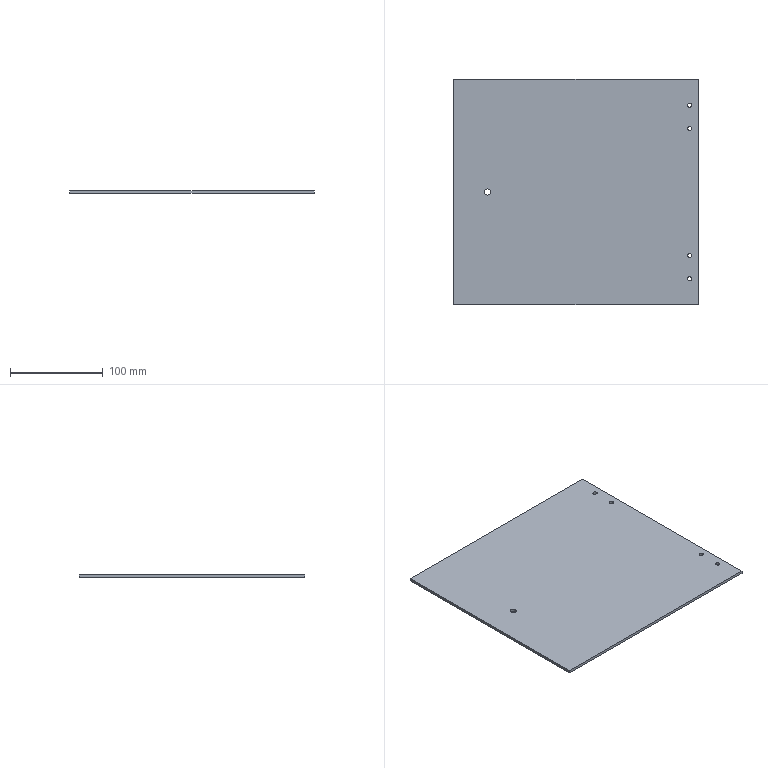Part | SolidWorks | features Cut 2, Extrusion 1, MirrorPattern 1 | 1 solid | 16 faces | box 263 x 243 x 3 mm | volume 191442 mm3 | cylinder 10 | plane 6 | commonest cylinder face diameters 4.4 x8 6.6 x2
STEP:
#1=CARTESIAN_POINT('',(-98.8,0.,0.));
#2=VERTEX_POINT('',#1);
#3=CARTESIAN_POINT('',(-92.2,0.,0.));
#4=VERTEX_POINT('',#3);
#5=CARTESIAN_POINT('',(-95.5,0.,0.));
#6=DIRECTION('',(0.,0.,1.));
#7=DIRECTION('',(1.,0.,0.));
#8=AXIS2_PLACEMENT_3D('',#5,#6,#7);
#9=CIRCLE('',#8,3.3);
#10=EDGE_CURVE('',#2,#4,#9,.T.);
#11=ORIENTED_EDGE('',*,*,#10,.F.);
#12=CARTESIAN_POINT('',(-98.8,0.,3.));
#13=VERTEX_POINT('',#12);
#14=CARTESIAN_POINT('',(-98.8,0.,-7.));
#15=DIRECTION('',(0.,0.,1.));
#16=VECTOR('',#15,1000.);
#17=LINE('',#14,#16);
#18=EDGE_CURVE('',#2,#13,#17,.T.);
#19=ORIENTED_EDGE('',*,*,#18,.T.);
#20=CARTESIAN_POINT('',(-92.2,0.,3.));
#21=VERTEX_POINT('',#20);
#22=CARTESIAN_POINT('',(-95.5,0.,3.));
#23=DIRECTION('',(0.,0.,1.));
#24=DIRECTION('',(1.,0.,0.));
#25=AXIS2_PLACEMENT_3D('',#22,#23,#24);
#26=CIRCLE('',#25,3.3);
#27=EDGE_CURVE('',#13,#21,#26,.T.);
#28=ORIENTED_EDGE('',*,*,#27,.T.);
#29=CARTESIAN_POINT('',(-92.2,0.,-7.));
#30=DIRECTION('',(0.,0.,1.));
#31=VECTOR('',#30,1000.);
#32=LINE('',#29,#31);
#33=EDGE_CURVE('',#4,#21,#32,.T.);
#34=ORIENTED_EDGE('',*,*,#33,.F.);
#35=EDGE_LOOP('',(#11,#19,#28,#34));
#36=FACE_OUTER_BOUND('',#35,.T.);
#37=CARTESIAN_POINT('',(-95.5,0.,-7.));
#38=DIRECTION('',(0.,0.,1.));
#39=DIRECTION('',(1.,0.,0.));
#40=AXIS2_PLACEMENT_3D('',#37,#38,#39);
#41=CYLINDRICAL_SURFACE('',#40,3.3);
#42=ADVANCED_FACE('',(#36),#41,.F.);
#43=CARTESIAN_POINT('',(124.7,68.5,3.));
#44=VERTEX_POINT('',#43);
#45=CARTESIAN_POINT('',(120.3,68.5,3.));
#46=VERTEX_POINT('',#45);
#47=CARTESIAN_POINT('',(122.5,68.5,3.));
#48=DIRECTION('',(0.,0.,-1.));
#49=DIRECTION('',(1.,0.,0.));
#50=AXIS2_PLACEMENT_3D('',#47,#48,#49);
#51=CIRCLE('',#50,2.2);
#52=EDGE_CURVE('',#44,#46,#51,.T.);
#53=ORIENTED_EDGE('',*,*,#52,.F.);
#54=CARTESIAN_POINT('',(124.7,68.5,0.));
#55=VERTEX_POINT('',#54);
#56=CARTESIAN_POINT('',(124.7,68.5,10.));
#57=DIRECTION('',(0.,0.,-1.));
#58=VECTOR('',#57,1000.);
#59=LINE('',#56,#58);
#60=EDGE_CURVE('',#44,#55,#59,.T.);
#61=ORIENTED_EDGE('',*,*,#60,.T.);
#62=CARTESIAN_POINT('',(120.3,68.5,0.));
#63=VERTEX_POINT('',#62);
#64=CARTESIAN_POINT('',(122.5,68.5,0.));
#65=DIRECTION('',(0.,0.,1.));
#66=DIRECTION('',(-1.,0.,0.));
#67=AXIS2_PLACEMENT_3D('',#64,#65,#66);
#68=CIRCLE('',#67,2.2);
#69=EDGE_CURVE('',#63,#55,#68,.T.);
#70=ORIENTED_EDGE('',*,*,#69,.F.);
#71=CARTESIAN_POINT('',(120.3,68.5,10.));
#72=DIRECTION('',(0.,0.,-1.));
#73=VECTOR('',#72,1000.);
#74=LINE('',#71,#73);
#75=EDGE_CURVE('',#46,#63,#74,.T.);
#76=ORIENTED_EDGE('',*,*,#75,.F.);
#77=EDGE_LOOP('',(#53,#61,#70,#76));
#78=FACE_OUTER_BOUND('',#77,.T.);
#79=CARTESIAN_POINT('',(122.5,68.5,10.));
#80=DIRECTION('',(0.,0.,-1.));
#81=DIRECTION('',(-1.,0.,0.));
#82=AXIS2_PLACEMENT_3D('',#79,#80,#81);
#83=CYLINDRICAL_SURFACE('',#82,2.2);
#84=ADVANCED_FACE('',(#78),#83,.F.);
#85=CARTESIAN_POINT('',(124.7,93.5,3.));
#86=VERTEX_POINT('',#85);
#87=CARTESIAN_POINT('',(120.3,93.5,3.));
#88=VERTEX_POINT('',#87);
#89=CARTESIAN_POINT('',(122.5,93.5,3.));
#90=DIRECTION('',(0.,0.,-1.));
#91=DIRECTION('',(1.,0.,0.));
#92=AXIS2_PLACEMENT_3D('',#89,#90,#91);
#93=CIRCLE('',#92,2.2);
#94=EDGE_CURVE('',#86,#88,#93,.T.);
#95=ORIENTED_EDGE('',*,*,#94,.F.);
#96=CARTESIAN_POINT('',(124.7,93.5,0.));
#97=VERTEX_POINT('',#96);
#98=CARTESIAN_POINT('',(124.7,93.5,10.));
#99=DIRECTION('',(0.,0.,-1.));
#100=VECTOR('',#99,1000.);
#101=LINE('',#98,#100);
#102=EDGE_CURVE('',#86,#97,#101,.T.);
#103=ORIENTED_EDGE('',*,*,#102,.T.);
#104=CARTESIAN_POINT('',(120.3,93.5,0.));
#105=VERTEX_POINT('',#104);
#106=CARTESIAN_POINT('',(122.5,93.5,0.));
#107=DIRECTION('',(0.,0.,1.));
#108=DIRECTION('',(-1.,0.,0.));
#109=AXIS2_PLACEMENT_3D('',#106,#107,#108);
#110=CIRCLE('',#109,2.2);
#111=EDGE_CURVE('',#105,#97,#110,.T.);
#112=ORIENTED_EDGE('',*,*,#111,.F.);
#113=CARTESIAN_POINT('',(120.3,93.5,10.));
#114=DIRECTION('',(0.,0.,-1.));
#115=VECTOR('',#114,1000.);
#116=LINE('',#113,#115);
#117=EDGE_CURVE('',#88,#105,#116,.T.);
#118=ORIENTED_EDGE('',*,*,#117,.F.);
#119=EDGE_LOOP('',(#95,#103,#112,#118));
#120=FACE_OUTER_BOUND('',#119,.T.);
#121=CARTESIAN_POINT('',(122.5,93.5,10.));
#122=DIRECTION('',(0.,0.,-1.));
#123=DIRECTION('',(-1.,0.,0.));
#124=AXIS2_PLACEMENT_3D('',#121,#122,#123);
#125=CYLINDRICAL_SURFACE('',#124,2.2);
#126=ADVANCED_FACE('',(#120),#125,.F.);
#127=CARTESIAN_POINT('',(120.3,-68.5,3.));
#128=VERTEX_POINT('',#127);
#129=CARTESIAN_POINT('',(124.7,-68.5,3.));
#130=VERTEX_POINT('',#129);
#131=CARTESIAN_POINT('',(122.5,-68.5,3.));
#132=DIRECTION('',(0.,0.,1.));
#133=DIRECTION('',(1.,0.,0.));
#134=AXIS2_PLACEMENT_3D('',#131,#132,#133);
#135=CIRCLE('',#134,2.2);
#136=EDGE_CURVE('',#128,#130,#135,.T.);
#137=ORIENTED_EDGE('',*,*,#136,.T.);
#138=CARTESIAN_POINT('',(124.7,-68.5,0.));
#139=VERTEX_POINT('',#138);
#140=CARTESIAN_POINT('',(124.7,-68.5,10.));
#141=DIRECTION('',(0.,0.,-1.));
#142=VECTOR('',#141,1000.);
#143=LINE('',#140,#142);
#144=EDGE_CURVE('',#130,#139,#143,.T.);
#145=ORIENTED_EDGE('',*,*,#144,.T.);
#146=CARTESIAN_POINT('',(120.3,-68.5,0.));
#147=VERTEX_POINT('',#146);
#148=CARTESIAN_POINT('',(122.5,-68.5,0.));
#149=DIRECTION('',(0.,0.,-1.));
#150=DIRECTION('',(-1.,0.,0.));
#151=AXIS2_PLACEMENT_3D('',#148,#149,#150);
#152=CIRCLE('',#151,2.2);
#153=EDGE_CURVE('',#139,#147,#152,.T.);
#154=ORIENTED_EDGE('',*,*,#153,.T.);
#155=CARTESIAN_POINT('',(120.3,-68.5,10.));
#156=DIRECTION('',(0.,0.,-1.));
#157=VECTOR('',#156,1000.);
#158=LINE('',#155,#157);
#159=EDGE_CURVE('',#128,#147,#158,.T.);
#160=ORIENTED_EDGE('',*,*,#159,.F.);
#161=EDGE_LOOP('',(#137,#145,#154,#160));
#162=FACE_OUTER_BOUND('',#161,.T.);
#163=CARTESIAN_POINT('',(122.5,-68.5,10.));
#164=DIRECTION('',(0.,0.,-1.));
#165=DIRECTION('',(-1.,0.,0.));
#166=AXIS2_PLACEMENT_3D('',#163,#164,#165);
#167=CYLINDRICAL_SURFACE('',#166,2.2);
#168=ADVANCED_FACE('',(#162),#167,.F.);
#169=CARTESIAN_POINT('',(120.3,-93.5,3.));
#170=VERTEX_POINT('',#169);
#171=CARTESIAN_POINT('',(124.7,-93.5,3.));
#172=VERTEX_POINT('',#171);
#173=CARTESIAN_POINT('',(122.5,-93.5,3.));
#174=DIRECTION('',(0.,0.,1.));
#175=DIRECTION('',(1.,0.,0.));
#176=AXIS2_PLACEMENT_3D('',#173,#174,#175);
#177=CIRCLE('',#176,2.2);
#178=EDGE_CURVE('',#170,#172,#177,.T.);
#179=ORIENTED_EDGE('',*,*,#178,.T.);
#180=CARTESIAN_POINT('',(124.7,-93.5,0.));
#181=VERTEX_POINT('',#180);
#182=CARTESIAN_POINT('',(124.7,-93.5,10.));
#183=DIRECTION('',(0.,0.,-1.));
#184=VECTOR('',#183,1000.);
#185=LINE('',#182,#184);
#186=EDGE_CURVE('',#172,#181,#185,.T.);
#187=ORIENTED_EDGE('',*,*,#186,.T.);
#188=CARTESIAN_POINT('',(120.3,-93.5,0.));
#189=VERTEX_POINT('',#188);
#190=CARTESIAN_POINT('',(122.5,-93.5,0.));
#191=DIRECTION('',(0.,0.,-1.));
#192=DIRECTION('',(-1.,0.,0.));
#193=AXIS2_PLACEMENT_3D('',#190,#191,#192);
#194=CIRCLE('',#193,2.2);
#195=EDGE_CURVE('',#181,#189,#194,.T.);
#196=ORIENTED_EDGE('',*,*,#195,.T.);
#197=CARTESIAN_POINT('',(120.3,-93.5,10.));
#198=DIRECTION('',(0.,0.,-1.));
#199=VECTOR('',#198,1000.);
#200=LINE('',#197,#199);
#201=EDGE_CURVE('',#170,#189,#200,.T.);
#202=ORIENTED_EDGE('',*,*,#201,.F.);
#203=EDGE_LOOP('',(#179,#187,#196,#202));
#204=FACE_OUTER_BOUND('',#203,.T.);
#205=CARTESIAN_POINT('',(122.5,-93.5,10.));
#206=DIRECTION('',(0.,0.,-1.));
#207=DIRECTION('',(-1.,0.,0.));
#208=AXIS2_PLACEMENT_3D('',#205,#206,#207);
#209=CYLINDRICAL_SURFACE('',#208,2.2);
#210=ADVANCED_FACE('',(#204),#209,.F.);
#211=CARTESIAN_POINT('',(-131.5,121.5,0.));
#212=VERTEX_POINT('',#211);
#213=CARTESIAN_POINT('',(-131.5,-121.5,0.));
#214=VERTEX_POINT('',#213);
#215=CARTESIAN_POINT('',(-131.5,-121.5,0.));
#216=DIRECTION('',(0.,-1.,0.));
#217=VECTOR('',#216,1000.);
#218=LINE('',#215,#217);
#219=EDGE_CURVE('',#212,#214,#218,.T.);
#220=ORIENTED_EDGE('',*,*,#219,.T.);
#221=CARTESIAN_POINT('',(-131.5,-121.5,3.));
#222=VERTEX_POINT('',#221);
#223=CARTESIAN_POINT('',(-131.5,-121.5,3.));
#224=DIRECTION('',(0.,0.,-1.));
#225=VECTOR('',#224,1000.);
#226=LINE('',#223,#225);
#227=EDGE_CURVE('',#222,#214,#226,.T.);
#228=ORIENTED_EDGE('',*,*,#227,.F.);
#229=CARTESIAN_POINT('',(-131.5,121.5,3.));
#230=VERTEX_POINT('',#229);
#231=CARTESIAN_POINT('',(-131.5,-121.5,3.));
#232=DIRECTION('',(0.,-1.,0.));
#233=VECTOR('',#232,1000.);
#234=LINE('',#231,#233);
#235=EDGE_CURVE('',#230,#222,#234,.T.);
#236=ORIENTED_EDGE('',*,*,#235,.F.);
#237=CARTESIAN_POINT('',(-131.5,121.5,3.));
#238=DIRECTION('',(0.,0.,-1.));
#239=VECTOR('',#238,1000.);
#240=LINE('',#237,#239);
#241=EDGE_CURVE('',#230,#212,#240,.T.);
#242=ORIENTED_EDGE('',*,*,#241,.T.);
#243=EDGE_LOOP('',(#220,#228,#236,#242));
#244=FACE_OUTER_BOUND('',#243,.T.);
#245=CARTESIAN_POINT('',(-131.5,-121.5,3.));
#246=DIRECTION('',(1.,0.,0.));
#247=DIRECTION('',(0.,0.,-1.));
#248=AXIS2_PLACEMENT_3D('',#245,#246,#247);
#249=PLANE('',#248);
#250=ADVANCED_FACE('',(#244),#249,.F.);
#251=CARTESIAN_POINT('',(131.5,-121.5,0.));
#252=VERTEX_POINT('',#251);
#253=CARTESIAN_POINT('',(131.5,-121.5,0.));
#254=DIRECTION('',(1.,0.,0.));
#255=VECTOR('',#254,1000.);
#256=LINE('',#253,#255);
#257=EDGE_CURVE('',#214,#252,#256,.T.);
#258=ORIENTED_EDGE('',*,*,#257,.T.);
#259=CARTESIAN_POINT('',(131.5,-121.5,3.));
#260=VERTEX_POINT('',#259);
#261=CARTESIAN_POINT('',(131.5,-121.5,3.));
#262=DIRECTION('',(0.,0.,-1.));
#263=VECTOR('',#262,1000.);
#264=LINE('',#261,#263);
#265=EDGE_CURVE('',#260,#252,#264,.T.);
#266=ORIENTED_EDGE('',*,*,#265,.F.);
#267=CARTESIAN_POINT('',(131.5,-121.5,3.));
#268=DIRECTION('',(1.,0.,0.));
#269=VECTOR('',#268,1000.);
#270=LINE('',#267,#269);
#271=EDGE_CURVE('',#222,#260,#270,.T.);
#272=ORIENTED_EDGE('',*,*,#271,.F.);
#273=ORIENTED_EDGE('',*,*,#227,.T.);
#274=EDGE_LOOP('',(#258,#266,#272,#273));
#275=FACE_OUTER_BOUND('',#274,.T.);
#276=CARTESIAN_POINT('',(131.5,-121.5,3.));
#277=DIRECTION('',(0.,1.,0.));
#278=DIRECTION('',(-1.,0.,0.));
#279=AXIS2_PLACEMENT_3D('',#276,#277,#278);
#280=PLANE('',#279);
#281=ADVANCED_FACE('',(#275),#280,.F.);
#282=CARTESIAN_POINT('',(131.5,121.5,0.));
#283=VERTEX_POINT('',#282);
#284=CARTESIAN_POINT('',(131.5,-121.5,0.));
#285=DIRECTION('',(0.,1.,0.));
#286=VECTOR('',#285,1000.);
#287=LINE('',#284,#286);
#288=EDGE_CURVE('',#252,#283,#287,.T.);
#289=ORIENTED_EDGE('',*,*,#288,.T.);
#290=CARTESIAN_POINT('',(131.5,121.5,3.));
#291=VERTEX_POINT('',#290);
#292=CARTESIAN_POINT('',(131.5,121.5,3.));
#293=DIRECTION('',(0.,0.,-1.));
#294=VECTOR('',#293,1000.);
#295=LINE('',#292,#294);
#296=EDGE_CURVE('',#291,#283,#295,.T.);
#297=ORIENTED_EDGE('',*,*,#296,.F.);
#298=CARTESIAN_POINT('',(131.5,-121.5,3.));
#299=DIRECTION('',(0.,1.,0.));
#300=VECTOR('',#299,1000.);
#301=LINE('',#298,#300);
#302=EDGE_CURVE('',#260,#291,#301,.T.);
#303=ORIENTED_EDGE('',*,*,#302,.F.);
#304=ORIENTED_EDGE('',*,*,#265,.T.);
#305=EDGE_LOOP('',(#289,#297,#303,#304));
#306=FACE_OUTER_BOUND('',#305,.T.);
#307=CARTESIAN_POINT('',(131.5,-121.5,3.));
#308=DIRECTION('',(-1.,0.,0.));
#309=DIRECTION('',(0.,0.,1.));
#310=AXIS2_PLACEMENT_3D('',#307,#308,#309);
#311=PLANE('',#310);
#312=ADVANCED_FACE('',(#306),#311,.F.);
#313=CARTESIAN_POINT('',(131.5,121.5,0.));
#314=DIRECTION('',(-1.,0.,0.));
#315=VECTOR('',#314,1000.);
#316=LINE('',#313,#315);
#317=EDGE_CURVE('',#283,#212,#316,.T.);
#318=ORIENTED_EDGE('',*,*,#317,.T.);
#319=ORIENTED_EDGE('',*,*,#241,.F.);
#320=CARTESIAN_POINT('',(131.5,121.5,3.));
#321=DIRECTION('',(-1.,0.,0.));
#322=VECTOR('',#321,1000.);
#323=LINE('',#320,#322);
#324=EDGE_CURVE('',#291,#230,#323,.T.);
#325=ORIENTED_EDGE('',*,*,#324,.F.);
#326=ORIENTED_EDGE('',*,*,#296,.T.);
#327=EDGE_LOOP('',(#318,#319,#325,#326));
#328=FACE_OUTER_BOUND('',#327,.T.);
#329=CARTESIAN_POINT('',(131.5,121.5,3.));
#330=DIRECTION('',(0.,-1.,0.));
#331=DIRECTION('',(1.,0.,0.));
#332=AXIS2_PLACEMENT_3D('',#329,#330,#331);
#333=PLANE('',#332);
#334=ADVANCED_FACE('',(#328),#333,.F.);
#335=CARTESIAN_POINT('',(-95.5,0.,3.));
#336=DIRECTION('',(0.,0.,1.));
#337=DIRECTION('',(1.,0.,0.));
#338=AXIS2_PLACEMENT_3D('',#335,#336,#337);
#339=CIRCLE('',#338,3.3);
#340=EDGE_CURVE('',#21,#13,#339,.T.);
#341=ORIENTED_EDGE('',*,*,#340,.F.);
#342=ORIENTED_EDGE('',*,*,#27,.F.);
#343=EDGE_LOOP('',(#341,#342));
#344=FACE_BOUND('',#343,.T.);
#345=CARTESIAN_POINT('',(122.5,68.5,3.));
#346=DIRECTION('',(0.,0.,-1.));
#347=DIRECTION('',(1.,0.,0.));
#348=AXIS2_PLACEMENT_3D('',#345,#346,#347);
#349=CIRCLE('',#348,2.2);
#350=EDGE_CURVE('',#46,#44,#349,.T.);
#351=ORIENTED_EDGE('',*,*,#350,.T.);
#352=ORIENTED_EDGE('',*,*,#52,.T.);
#353=EDGE_LOOP('',(#351,#352));
#354=FACE_BOUND('',#353,.T.);
#355=CARTESIAN_POINT('',(122.5,93.5,3.));
#356=DIRECTION('',(0.,0.,-1.));
#357=DIRECTION('',(1.,0.,0.));
#358=AXIS2_PLACEMENT_3D('',#355,#356,#357);
#359=CIRCLE('',#358,2.2);
#360=EDGE_CURVE('',#88,#86,#359,.T.);
#361=ORIENTED_EDGE('',*,*,#360,.T.);
#362=ORIENTED_EDGE('',*,*,#94,.T.);
#363=EDGE_LOOP('',(#361,#362));
#364=FACE_BOUND('',#363,.T.);
#365=ORIENTED_EDGE('',*,*,#136,.F.);
#366=CARTESIAN_POINT('',(122.5,-68.5,3.));
#367=DIRECTION('',(0.,0.,1.));
#368=DIRECTION('',(1.,0.,0.));
#369=AXIS2_PLACEMENT_3D('',#366,#367,#368);
#370=CIRCLE('',#369,2.2);
#371=EDGE_CURVE('',#130,#128,#370,.T.);
#372=ORIENTED_EDGE('',*,*,#371,.F.);
#373=EDGE_LOOP('',(#365,#372));
#374=FACE_BOUND('',#373,.T.);
#375=ORIENTED_EDGE('',*,*,#178,.F.);
#376=CARTESIAN_POINT('',(122.5,-93.5,3.));
#377=DIRECTION('',(0.,0.,1.));
#378=DIRECTION('',(1.,0.,0.));
#379=AXIS2_PLACEMENT_3D('',#376,#377,#378);
#380=CIRCLE('',#379,2.2);
#381=EDGE_CURVE('',#172,#170,#380,.T.);
#382=ORIENTED_EDGE('',*,*,#381,.F.);
#383=EDGE_LOOP('',(#375,#382));
#384=FACE_BOUND('',#383,.T.);
#385=ORIENTED_EDGE('',*,*,#235,.T.);
#386=ORIENTED_EDGE('',*,*,#271,.T.);
#387=ORIENTED_EDGE('',*,*,#302,.T.);
#388=ORIENTED_EDGE('',*,*,#324,.T.);
#389=EDGE_LOOP('',(#385,#386,#387,#388));
#390=FACE_OUTER_BOUND('',#389,.T.);
#391=CARTESIAN_POINT('',(0.,0.,3.));
#392=DIRECTION('',(0.,0.,1.));
#393=DIRECTION('',(1.,0.,0.));
#394=AXIS2_PLACEMENT_3D('',#391,#392,#393);
#395=PLANE('',#394);
#396=ADVANCED_FACE('',(#344,#354,#364,#374,#384,#390),#395,.T.);
#397=CARTESIAN_POINT('',(-95.5,0.,0.));
#398=DIRECTION('',(0.,0.,1.));
#399=DIRECTION('',(1.,0.,0.));
#400=AXIS2_PLACEMENT_3D('',#397,#398,#399);
#401=CIRCLE('',#400,3.3);
#402=EDGE_CURVE('',#4,#2,#401,.T.);
#403=ORIENTED_EDGE('',*,*,#402,.T.);
#404=ORIENTED_EDGE('',*,*,#10,.T.);
#405=EDGE_LOOP('',(#403,#404));
#406=FACE_BOUND('',#405,.T.);
#407=ORIENTED_EDGE('',*,*,#69,.T.);
#408=CARTESIAN_POINT('',(122.5,68.5,0.));
#409=DIRECTION('',(0.,0.,1.));
#410=DIRECTION('',(-1.,0.,0.));
#411=AXIS2_PLACEMENT_3D('',#408,#409,#410);
#412=CIRCLE('',#411,2.2);
#413=EDGE_CURVE('',#55,#63,#412,.T.);
#414=ORIENTED_EDGE('',*,*,#413,.T.);
#415=EDGE_LOOP('',(#407,#414));
#416=FACE_BOUND('',#415,.T.);
#417=ORIENTED_EDGE('',*,*,#111,.T.);
#418=CARTESIAN_POINT('',(122.5,93.5,0.));
#419=DIRECTION('',(0.,0.,1.));
#420=DIRECTION('',(-1.,0.,0.));
#421=AXIS2_PLACEMENT_3D('',#418,#419,#420);
#422=CIRCLE('',#421,2.2);
#423=EDGE_CURVE('',#97,#105,#422,.T.);
#424=ORIENTED_EDGE('',*,*,#423,.T.);
#425=EDGE_LOOP('',(#417,#424));
#426=FACE_BOUND('',#425,.T.);
#427=CARTESIAN_POINT('',(122.5,-68.5,0.));
#428=DIRECTION('',(0.,0.,-1.));
#429=DIRECTION('',(-1.,0.,0.));
#430=AXIS2_PLACEMENT_3D('',#427,#428,#429);
#431=CIRCLE('',#430,2.2);
#432=EDGE_CURVE('',#147,#139,#431,.T.);
#433=ORIENTED_EDGE('',*,*,#432,.F.);
#434=ORIENTED_EDGE('',*,*,#153,.F.);
#435=EDGE_LOOP('',(#433,#434));
#436=FACE_BOUND('',#435,.T.);
#437=CARTESIAN_POINT('',(122.5,-93.5,0.));
#438=DIRECTION('',(0.,0.,-1.));
#439=DIRECTION('',(-1.,0.,0.));
#440=AXIS2_PLACEMENT_3D('',#437,#438,#439);
#441=CIRCLE('',#440,2.2);
#442=EDGE_CURVE('',#189,#181,#441,.T.);
#443=ORIENTED_EDGE('',*,*,#442,.F.);
#444=ORIENTED_EDGE('',*,*,#195,.F.);
#445=EDGE_LOOP('',(#443,#444));
#446=FACE_BOUND('',#445,.T.);
#447=ORIENTED_EDGE('',*,*,#219,.F.);
#448=ORIENTED_EDGE('',*,*,#317,.F.);
#449=ORIENTED_EDGE('',*,*,#288,.F.);
#450=ORIENTED_EDGE('',*,*,#257,.F.);
#451=EDGE_LOOP('',(#447,#448,#449,#450));
#452=FACE_OUTER_BOUND('',#451,.T.);
#453=CARTESIAN_POINT('',(0.,0.,0.));
#454=DIRECTION('',(0.,0.,1.));
#455=DIRECTION('',(1.,0.,0.));
#456=AXIS2_PLACEMENT_3D('',#453,#454,#455);
#457=PLANE('',#456);
#458=ADVANCED_FACE('',(#406,#416,#426,#436,#446,#452),#457,.F.);
#459=ORIENTED_EDGE('',*,*,#186,.F.);
#460=ORIENTED_EDGE('',*,*,#381,.T.);
#461=ORIENTED_EDGE('',*,*,#201,.T.);
#462=ORIENTED_EDGE('',*,*,#442,.T.);
#463=EDGE_LOOP('',(#459,#460,#461,#462));
#464=FACE_OUTER_BOUND('',#463,.T.);
#465=CARTESIAN_POINT('',(122.5,-93.5,10.));
#466=DIRECTION('',(0.,0.,-1.));
#467=DIRECTION('',(-1.,0.,0.));
#468=AXIS2_PLACEMENT_3D('',#465,#466,#467);
#469=CYLINDRICAL_SURFACE('',#468,2.2);
#470=ADVANCED_FACE('',(#464),#469,.F.);
#471=ORIENTED_EDGE('',*,*,#144,.F.);
#472=ORIENTED_EDGE('',*,*,#371,.T.);
#473=ORIENTED_EDGE('',*,*,#159,.T.);
#474=ORIENTED_EDGE('',*,*,#432,.T.);
#475=EDGE_LOOP('',(#471,#472,#473,#474));
#476=FACE_OUTER_BOUND('',#475,.T.);
#477=CARTESIAN_POINT('',(122.5,-68.5,10.));
#478=DIRECTION('',(0.,0.,-1.));
#479=DIRECTION('',(-1.,0.,0.));
#480=AXIS2_PLACEMENT_3D('',#477,#478,#479);
#481=CYLINDRICAL_SURFACE('',#480,2.2);
#482=ADVANCED_FACE('',(#476),#481,.F.);
#483=ORIENTED_EDGE('',*,*,#102,.F.);
#484=ORIENTED_EDGE('',*,*,#360,.F.);
#485=ORIENTED_EDGE('',*,*,#117,.T.);
#486=ORIENTED_EDGE('',*,*,#423,.F.);
#487=EDGE_LOOP('',(#483,#484,#485,#486));
#488=FACE_OUTER_BOUND('',#487,.T.);
#489=CARTESIAN_POINT('',(122.5,93.5,10.));
#490=DIRECTION('',(0.,0.,-1.));
#491=DIRECTION('',(-1.,0.,0.));
#492=AXIS2_PLACEMENT_3D('',#489,#490,#491);
#493=CYLINDRICAL_SURFACE('',#492,2.2);
#494=ADVANCED_FACE('',(#488),#493,.F.);
#495=ORIENTED_EDGE('',*,*,#60,.F.);
#496=ORIENTED_EDGE('',*,*,#350,.F.);
#497=ORIENTED_EDGE('',*,*,#75,.T.);
#498=ORIENTED_EDGE('',*,*,#413,.F.);
#499=EDGE_LOOP('',(#495,#496,#497,#498));
#500=FACE_OUTER_BOUND('',#499,.T.);
#501=CARTESIAN_POINT('',(122.5,68.5,10.));
#502=DIRECTION('',(0.,0.,-1.));
#503=DIRECTION('',(-1.,0.,0.));
#504=AXIS2_PLACEMENT_3D('',#501,#502,#503);
#505=CYLINDRICAL_SURFACE('',#504,2.2);
#506=ADVANCED_FACE('',(#500),#505,.F.);
#507=ORIENTED_EDGE('',*,*,#18,.F.);
#508=ORIENTED_EDGE('',*,*,#402,.F.);
#509=ORIENTED_EDGE('',*,*,#33,.T.);
#510=ORIENTED_EDGE('',*,*,#340,.T.);
#511=EDGE_LOOP('',(#507,#508,#509,#510));
#512=FACE_OUTER_BOUND('',#511,.T.);
#513=CARTESIAN_POINT('',(-95.5,0.,-7.));
#514=DIRECTION('',(0.,0.,1.));
#515=DIRECTION('',(1.,0.,0.));
#516=AXIS2_PLACEMENT_3D('',#513,#514,#515);
#517=CYLINDRICAL_SURFACE('',#516,3.3);
#518=ADVANCED_FACE('',(#512),#517,.F.);
#519=CLOSED_SHELL('',(#42,#84,#126,#168,#210,#250,#281,#312,#334,#396,#458,#470,#482,#494,#506,#518));
#520=MANIFOLD_SOLID_BREP('',#519);
#521=CARTESIAN_POINT('',(0.,0.,0.));
#522=DIRECTION('',(0.,0.,1.));
#523=DIRECTION('',(1.,0.,0.));
#524=AXIS2_PLACEMENT_3D('',#521,#522,#523);
#525=(LENGTH_UNIT()NAMED_UNIT(*)SI_UNIT(.MILLI.,.METRE.));
#526=UNCERTAINTY_MEASURE_WITH_UNIT(LENGTH_MEASURE(0.00001),#525,'','');
#527=(NAMED_UNIT(*)PLANE_ANGLE_UNIT()SI_UNIT($,.RADIAN.));
#528=(NAMED_UNIT(*)SI_UNIT($,.STERADIAN.)SOLID_ANGLE_UNIT());
#529=(GEOMETRIC_REPRESENTATION_CONTEXT(3)GLOBAL_UNCERTAINTY_ASSIGNED_CONTEXT((#526))GLOBAL_UNIT_ASSIGNED_CONTEXT((#525,#527,#528))REPRESENTATION_CONTEXT('',''));
#530=ADVANCED_BREP_SHAPE_REPRESENTATION('',(#520,#524),#529);